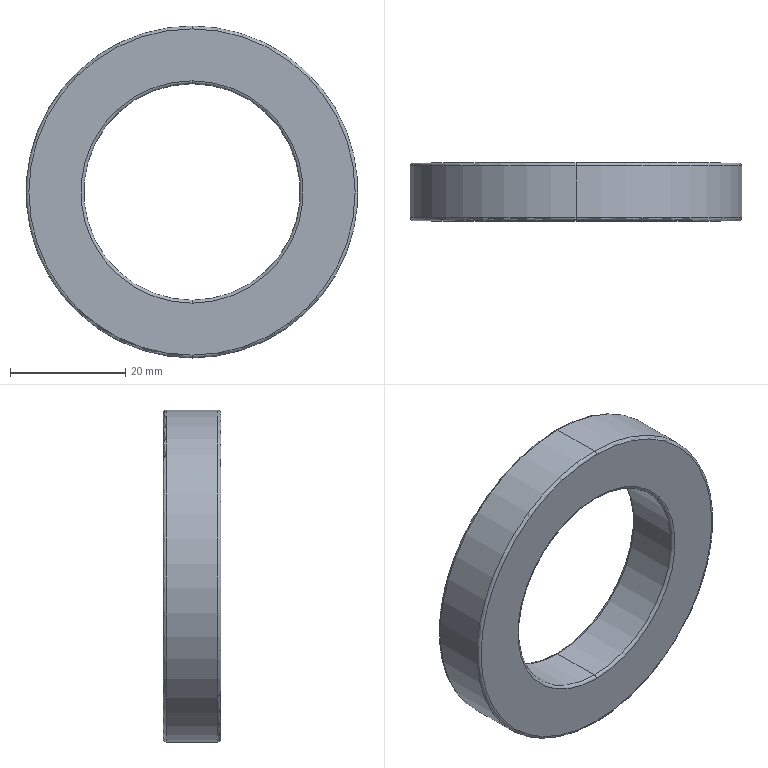Part | STEP file | 2026.6.15-Main Assembly图.sldasm-Part-131 | 1 solid | 14 faces | box 57.5 x 10 x 57.5 mm | volume 14891 mm3 | torus 8 | cylinder 4 | plane 2 | commonest cylinder face diameters 37.5 x2 57.5 x2
STEP:
#1=CARTESIAN_POINT('',(-1589.224,502.551,4179.917));
#2=VERTEX_POINT('',#1);
#3=CARTESIAN_POINT('',(-1589.224,502.551,4237.417));
#4=VERTEX_POINT('',#3);
#5=CARTESIAN_POINT('',(-1589.224,502.551,4208.667));
#6=DIRECTION('',(0.,-1.,0.));
#7=DIRECTION('',(0.,0.,1.));
#8=AXIS2_PLACEMENT_3D('',#5,#6,#7);
#9=CIRCLE('',#8,28.75);
#10=EDGE_CURVE('',#2,#4,#9,.T.);
#11=ORIENTED_EDGE('',*,*,#10,.F.);
#12=CARTESIAN_POINT('',(-1589.224,503.051,4180.417));
#13=VERTEX_POINT('',#12);
#14=CARTESIAN_POINT('',(-1589.224,502.551,4180.417));
#15=DIRECTION('',(1.,0.,0.));
#16=DIRECTION('',(0.,0.,-1.));
#17=AXIS2_PLACEMENT_3D('',#14,#15,#16);
#18=CIRCLE('',#17,0.5);
#19=EDGE_CURVE('',#2,#13,#18,.T.);
#20=ORIENTED_EDGE('',*,*,#19,.T.);
#21=CARTESIAN_POINT('',(-1589.224,503.051,4236.917));
#22=VERTEX_POINT('',#21);
#23=CARTESIAN_POINT('',(-1589.224,503.051,4208.667));
#24=DIRECTION('',(0.,1.,0.));
#25=DIRECTION('',(0.,0.,1.));
#26=AXIS2_PLACEMENT_3D('',#23,#24,#25);
#27=CIRCLE('',#26,28.25);
#28=EDGE_CURVE('',#22,#13,#27,.T.);
#29=ORIENTED_EDGE('',*,*,#28,.F.);
#30=CARTESIAN_POINT('',(-1589.224,502.551,4236.917));
#31=DIRECTION('',(-1.,0.,0.));
#32=DIRECTION('',(0.,0.,1.));
#33=AXIS2_PLACEMENT_3D('',#30,#31,#32);
#34=CIRCLE('',#33,0.5);
#35=EDGE_CURVE('',#4,#22,#34,.T.);
#36=ORIENTED_EDGE('',*,*,#35,.F.);
#37=EDGE_LOOP('',(#11,#20,#29,#36));
#38=FACE_OUTER_BOUND('',#37,.T.);
#39=CARTESIAN_POINT('',(-1589.224,502.551,4208.667));
#40=DIRECTION('',(0.,1.,0.));
#41=DIRECTION('',(0.,0.,1.));
#42=AXIS2_PLACEMENT_3D('',#39,#40,#41);
#43=TOROIDAL_SURFACE('',#42,28.25,0.5);
#44=ADVANCED_FACE('',(#38),#43,.T.);
#45=CARTESIAN_POINT('',(-1589.224,503.051,4189.417));
#46=VERTEX_POINT('',#45);
#47=CARTESIAN_POINT('',(-1589.224,503.051,4227.917));
#48=VERTEX_POINT('',#47);
#49=CARTESIAN_POINT('',(-1589.224,503.051,4208.667));
#50=DIRECTION('',(0.,-1.,0.));
#51=DIRECTION('',(0.,0.,1.));
#52=AXIS2_PLACEMENT_3D('',#49,#50,#51);
#53=CIRCLE('',#52,19.25);
#54=EDGE_CURVE('',#46,#48,#53,.T.);
#55=ORIENTED_EDGE('',*,*,#54,.F.);
#56=CARTESIAN_POINT('',(-1589.224,502.551,4189.917));
#57=VERTEX_POINT('',#56);
#58=CARTESIAN_POINT('',(-1589.224,502.551,4189.417));
#59=DIRECTION('',(1.,0.,0.));
#60=DIRECTION('',(0.,0.,-1.));
#61=AXIS2_PLACEMENT_3D('',#58,#59,#60);
#62=CIRCLE('',#61,0.5);
#63=EDGE_CURVE('',#46,#57,#62,.T.);
#64=ORIENTED_EDGE('',*,*,#63,.T.);
#65=CARTESIAN_POINT('',(-1589.224,502.551,4227.417));
#66=VERTEX_POINT('',#65);
#67=CARTESIAN_POINT('',(-1589.224,502.551,4208.667));
#68=DIRECTION('',(0.,1.,0.));
#69=DIRECTION('',(0.,0.,1.));
#70=AXIS2_PLACEMENT_3D('',#67,#68,#69);
#71=CIRCLE('',#70,18.75);
#72=EDGE_CURVE('',#66,#57,#71,.T.);
#73=ORIENTED_EDGE('',*,*,#72,.F.);
#74=CARTESIAN_POINT('',(-1589.224,502.551,4227.917));
#75=DIRECTION('',(-1.,0.,0.));
#76=DIRECTION('',(0.,0.,1.));
#77=AXIS2_PLACEMENT_3D('',#74,#75,#76);
#78=CIRCLE('',#77,0.5);
#79=EDGE_CURVE('',#48,#66,#78,.T.);
#80=ORIENTED_EDGE('',*,*,#79,.F.);
#81=EDGE_LOOP('',(#55,#64,#73,#80));
#82=FACE_OUTER_BOUND('',#81,.T.);
#83=CARTESIAN_POINT('',(-1589.224,502.551,4208.667));
#84=DIRECTION('',(0.,1.,0.));
#85=DIRECTION('',(0.,0.,1.));
#86=AXIS2_PLACEMENT_3D('',#83,#84,#85);
#87=TOROIDAL_SURFACE('',#86,19.25,0.5);
#88=ADVANCED_FACE('',(#82),#87,.T.);
#89=CARTESIAN_POINT('',(-1589.224,493.051,4227.917));
#90=VERTEX_POINT('',#89);
#91=CARTESIAN_POINT('',(-1589.224,493.051,4189.417));
#92=VERTEX_POINT('',#91);
#93=CARTESIAN_POINT('',(-1589.224,493.051,4208.667));
#94=DIRECTION('',(0.,1.,0.));
#95=DIRECTION('',(0.,0.,-1.));
#96=AXIS2_PLACEMENT_3D('',#93,#94,#95);
#97=CIRCLE('',#96,19.25);
#98=EDGE_CURVE('',#90,#92,#97,.T.);
#99=ORIENTED_EDGE('',*,*,#98,.F.);
#100=CARTESIAN_POINT('',(-1589.224,493.551,4227.417));
#101=VERTEX_POINT('',#100);
#102=CARTESIAN_POINT('',(-1589.224,493.551,4227.917));
#103=DIRECTION('',(1.,0.,0.));
#104=DIRECTION('',(0.,0.,-1.));
#105=AXIS2_PLACEMENT_3D('',#102,#103,#104);
#106=CIRCLE('',#105,0.5);
#107=EDGE_CURVE('',#90,#101,#106,.T.);
#108=ORIENTED_EDGE('',*,*,#107,.T.);
#109=CARTESIAN_POINT('',(-1589.224,493.551,4189.917));
#110=VERTEX_POINT('',#109);
#111=CARTESIAN_POINT('',(-1589.224,493.551,4208.667));
#112=DIRECTION('',(0.,-1.,0.));
#113=DIRECTION('',(0.,0.,-1.));
#114=AXIS2_PLACEMENT_3D('',#111,#112,#113);
#115=CIRCLE('',#114,18.75);
#116=EDGE_CURVE('',#110,#101,#115,.T.);
#117=ORIENTED_EDGE('',*,*,#116,.F.);
#118=CARTESIAN_POINT('',(-1589.224,493.551,4189.417));
#119=DIRECTION('',(-1.,0.,0.));
#120=DIRECTION('',(0.,0.,1.));
#121=AXIS2_PLACEMENT_3D('',#118,#119,#120);
#122=CIRCLE('',#121,0.5);
#123=EDGE_CURVE('',#92,#110,#122,.T.);
#124=ORIENTED_EDGE('',*,*,#123,.F.);
#125=EDGE_LOOP('',(#99,#108,#117,#124));
#126=FACE_OUTER_BOUND('',#125,.T.);
#127=CARTESIAN_POINT('',(-1589.224,493.551,4208.667));
#128=DIRECTION('',(0.,-1.,0.));
#129=DIRECTION('',(0.,0.,-1.));
#130=AXIS2_PLACEMENT_3D('',#127,#128,#129);
#131=TOROIDAL_SURFACE('',#130,19.25,0.5);
#132=ADVANCED_FACE('',(#126),#131,.T.);
#133=CARTESIAN_POINT('',(-1589.224,493.551,4237.417));
#134=VERTEX_POINT('',#133);
#135=CARTESIAN_POINT('',(-1589.224,493.551,4179.917));
#136=VERTEX_POINT('',#135);
#137=CARTESIAN_POINT('',(-1589.224,493.551,4208.667));
#138=DIRECTION('',(0.,1.,0.));
#139=DIRECTION('',(0.,0.,-1.));
#140=AXIS2_PLACEMENT_3D('',#137,#138,#139);
#141=CIRCLE('',#140,28.75);
#142=EDGE_CURVE('',#134,#136,#141,.T.);
#143=ORIENTED_EDGE('',*,*,#142,.F.);
#144=CARTESIAN_POINT('',(-1589.224,493.051,4236.917));
#145=VERTEX_POINT('',#144);
#146=CARTESIAN_POINT('',(-1589.224,493.551,4236.917));
#147=DIRECTION('',(1.,0.,0.));
#148=DIRECTION('',(0.,0.,-1.));
#149=AXIS2_PLACEMENT_3D('',#146,#147,#148);
#150=CIRCLE('',#149,0.5);
#151=EDGE_CURVE('',#134,#145,#150,.T.);
#152=ORIENTED_EDGE('',*,*,#151,.T.);
#153=CARTESIAN_POINT('',(-1589.224,493.051,4180.417));
#154=VERTEX_POINT('',#153);
#155=CARTESIAN_POINT('',(-1589.224,493.051,4208.667));
#156=DIRECTION('',(0.,-1.,0.));
#157=DIRECTION('',(0.,0.,-1.));
#158=AXIS2_PLACEMENT_3D('',#155,#156,#157);
#159=CIRCLE('',#158,28.25);
#160=EDGE_CURVE('',#154,#145,#159,.T.);
#161=ORIENTED_EDGE('',*,*,#160,.F.);
#162=CARTESIAN_POINT('',(-1589.224,493.551,4180.417));
#163=DIRECTION('',(-1.,0.,0.));
#164=DIRECTION('',(0.,0.,1.));
#165=AXIS2_PLACEMENT_3D('',#162,#163,#164);
#166=CIRCLE('',#165,0.5);
#167=EDGE_CURVE('',#136,#154,#166,.T.);
#168=ORIENTED_EDGE('',*,*,#167,.F.);
#169=EDGE_LOOP('',(#143,#152,#161,#168));
#170=FACE_OUTER_BOUND('',#169,.T.);
#171=CARTESIAN_POINT('',(-1589.224,493.551,4208.667));
#172=DIRECTION('',(0.,-1.,0.));
#173=DIRECTION('',(0.,0.,-1.));
#174=AXIS2_PLACEMENT_3D('',#171,#172,#173);
#175=TOROIDAL_SURFACE('',#174,28.25,0.5);
#176=ADVANCED_FACE('',(#170),#175,.T.);
#177=CARTESIAN_POINT('',(-1589.224,493.551,4208.667));
#178=DIRECTION('',(0.,-1.,0.));
#179=DIRECTION('',(0.,0.,-1.));
#180=AXIS2_PLACEMENT_3D('',#177,#178,#179);
#181=CIRCLE('',#180,18.75);
#182=EDGE_CURVE('',#101,#110,#181,.T.);
#183=ORIENTED_EDGE('',*,*,#182,.T.);
#184=CARTESIAN_POINT('',(-1589.224,493.051,4189.917));
#185=DIRECTION('',(0.,1.,0.));
#186=VECTOR('',#185,1000.);
#187=LINE('',#184,#186);
#188=EDGE_CURVE('',#110,#57,#187,.T.);
#189=ORIENTED_EDGE('',*,*,#188,.T.);
#190=CARTESIAN_POINT('',(-1589.224,502.551,4208.667));
#191=DIRECTION('',(0.,1.,0.));
#192=DIRECTION('',(0.,0.,1.));
#193=AXIS2_PLACEMENT_3D('',#190,#191,#192);
#194=CIRCLE('',#193,18.75);
#195=EDGE_CURVE('',#57,#66,#194,.T.);
#196=ORIENTED_EDGE('',*,*,#195,.T.);
#197=CARTESIAN_POINT('',(-1589.224,493.051,4227.417));
#198=DIRECTION('',(0.,1.,0.));
#199=VECTOR('',#198,1000.);
#200=LINE('',#197,#199);
#201=EDGE_CURVE('',#101,#66,#200,.T.);
#202=ORIENTED_EDGE('',*,*,#201,.F.);
#203=EDGE_LOOP('',(#183,#189,#196,#202));
#204=FACE_OUTER_BOUND('',#203,.T.);
#205=CARTESIAN_POINT('',(-1589.224,493.051,4208.667));
#206=DIRECTION('',(0.,1.,0.));
#207=DIRECTION('',(0.,0.,1.));
#208=AXIS2_PLACEMENT_3D('',#205,#206,#207);
#209=CYLINDRICAL_SURFACE('',#208,18.75);
#210=ADVANCED_FACE('',(#204),#209,.F.);
#211=ORIENTED_EDGE('',*,*,#142,.T.);
#212=CARTESIAN_POINT('',(-1589.224,493.051,4179.917));
#213=DIRECTION('',(0.,1.,0.));
#214=VECTOR('',#213,1000.);
#215=LINE('',#212,#214);
#216=EDGE_CURVE('',#136,#2,#215,.T.);
#217=ORIENTED_EDGE('',*,*,#216,.T.);
#218=ORIENTED_EDGE('',*,*,#10,.T.);
#219=CARTESIAN_POINT('',(-1589.224,493.051,4237.417));
#220=DIRECTION('',(0.,1.,0.));
#221=VECTOR('',#220,1000.);
#222=LINE('',#219,#221);
#223=EDGE_CURVE('',#134,#4,#222,.T.);
#224=ORIENTED_EDGE('',*,*,#223,.F.);
#225=EDGE_LOOP('',(#211,#217,#218,#224));
#226=FACE_OUTER_BOUND('',#225,.T.);
#227=CARTESIAN_POINT('',(-1589.224,493.051,4208.667));
#228=DIRECTION('',(0.,1.,0.));
#229=DIRECTION('',(0.,0.,1.));
#230=AXIS2_PLACEMENT_3D('',#227,#228,#229);
#231=CYLINDRICAL_SURFACE('',#230,28.75);
#232=ADVANCED_FACE('',(#226),#231,.T.);
#233=CARTESIAN_POINT('',(-1589.224,503.051,4208.667));
#234=DIRECTION('',(0.,-1.,0.));
#235=DIRECTION('',(0.,0.,1.));
#236=AXIS2_PLACEMENT_3D('',#233,#234,#235);
#237=CIRCLE('',#236,19.25);
#238=EDGE_CURVE('',#48,#46,#237,.T.);
#239=ORIENTED_EDGE('',*,*,#238,.T.);
#240=ORIENTED_EDGE('',*,*,#54,.T.);
#241=EDGE_LOOP('',(#239,#240));
#242=FACE_BOUND('',#241,.T.);
#243=ORIENTED_EDGE('',*,*,#28,.T.);
#244=CARTESIAN_POINT('',(-1589.224,503.051,4208.667));
#245=DIRECTION('',(0.,1.,0.));
#246=DIRECTION('',(0.,0.,1.));
#247=AXIS2_PLACEMENT_3D('',#244,#245,#246);
#248=CIRCLE('',#247,28.25);
#249=EDGE_CURVE('',#13,#22,#248,.T.);
#250=ORIENTED_EDGE('',*,*,#249,.T.);
#251=EDGE_LOOP('',(#243,#250));
#252=FACE_OUTER_BOUND('',#251,.T.);
#253=CARTESIAN_POINT('',(-1589.224,503.051,4208.667));
#254=DIRECTION('',(0.,1.,0.));
#255=DIRECTION('',(0.,0.,1.));
#256=AXIS2_PLACEMENT_3D('',#253,#254,#255);
#257=PLANE('',#256);
#258=ADVANCED_FACE('',(#242,#252),#257,.T.);
#259=ORIENTED_EDGE('',*,*,#160,.T.);
#260=CARTESIAN_POINT('',(-1589.224,493.051,4208.667));
#261=DIRECTION('',(0.,-1.,0.));
#262=DIRECTION('',(0.,0.,-1.));
#263=AXIS2_PLACEMENT_3D('',#260,#261,#262);
#264=CIRCLE('',#263,28.25);
#265=EDGE_CURVE('',#145,#154,#264,.T.);
#266=ORIENTED_EDGE('',*,*,#265,.T.);
#267=EDGE_LOOP('',(#259,#266));
#268=FACE_OUTER_BOUND('',#267,.T.);
#269=CARTESIAN_POINT('',(-1589.224,493.051,4208.667));
#270=DIRECTION('',(0.,1.,0.));
#271=DIRECTION('',(0.,0.,-1.));
#272=AXIS2_PLACEMENT_3D('',#269,#270,#271);
#273=CIRCLE('',#272,19.25);
#274=EDGE_CURVE('',#92,#90,#273,.T.);
#275=ORIENTED_EDGE('',*,*,#274,.T.);
#276=ORIENTED_EDGE('',*,*,#98,.T.);
#277=EDGE_LOOP('',(#275,#276));
#278=FACE_BOUND('',#277,.T.);
#279=CARTESIAN_POINT('',(-1589.224,493.051,4208.667));
#280=DIRECTION('',(0.,-1.,0.));
#281=DIRECTION('',(0.,0.,-1.));
#282=AXIS2_PLACEMENT_3D('',#279,#280,#281);
#283=PLANE('',#282);
#284=ADVANCED_FACE('',(#268,#278),#283,.T.);
#285=ORIENTED_EDGE('',*,*,#216,.F.);
#286=CARTESIAN_POINT('',(-1589.224,493.551,4208.667));
#287=DIRECTION('',(0.,1.,0.));
#288=DIRECTION('',(0.,0.,-1.));
#289=AXIS2_PLACEMENT_3D('',#286,#287,#288);
#290=CIRCLE('',#289,28.75);
#291=EDGE_CURVE('',#136,#134,#290,.T.);
#292=ORIENTED_EDGE('',*,*,#291,.T.);
#293=ORIENTED_EDGE('',*,*,#223,.T.);
#294=CARTESIAN_POINT('',(-1589.224,502.551,4208.667));
#295=DIRECTION('',(0.,-1.,0.));
#296=DIRECTION('',(0.,0.,1.));
#297=AXIS2_PLACEMENT_3D('',#294,#295,#296);
#298=CIRCLE('',#297,28.75);
#299=EDGE_CURVE('',#4,#2,#298,.T.);
#300=ORIENTED_EDGE('',*,*,#299,.T.);
#301=EDGE_LOOP('',(#285,#292,#293,#300));
#302=FACE_OUTER_BOUND('',#301,.T.);
#303=CARTESIAN_POINT('',(-1589.224,493.051,4208.667));
#304=DIRECTION('',(0.,1.,0.));
#305=DIRECTION('',(0.,0.,1.));
#306=AXIS2_PLACEMENT_3D('',#303,#304,#305);
#307=CYLINDRICAL_SURFACE('',#306,28.75);
#308=ADVANCED_FACE('',(#302),#307,.T.);
#309=ORIENTED_EDGE('',*,*,#188,.F.);
#310=ORIENTED_EDGE('',*,*,#116,.T.);
#311=ORIENTED_EDGE('',*,*,#201,.T.);
#312=ORIENTED_EDGE('',*,*,#72,.T.);
#313=EDGE_LOOP('',(#309,#310,#311,#312));
#314=FACE_OUTER_BOUND('',#313,.T.);
#315=CARTESIAN_POINT('',(-1589.224,493.051,4208.667));
#316=DIRECTION('',(0.,1.,0.));
#317=DIRECTION('',(0.,0.,1.));
#318=AXIS2_PLACEMENT_3D('',#315,#316,#317);
#319=CYLINDRICAL_SURFACE('',#318,18.75);
#320=ADVANCED_FACE('',(#314),#319,.F.);
#321=ORIENTED_EDGE('',*,*,#151,.F.);
#322=ORIENTED_EDGE('',*,*,#291,.F.);
#323=ORIENTED_EDGE('',*,*,#167,.T.);
#324=ORIENTED_EDGE('',*,*,#265,.F.);
#325=EDGE_LOOP('',(#321,#322,#323,#324));
#326=FACE_OUTER_BOUND('',#325,.T.);
#327=CARTESIAN_POINT('',(-1589.224,493.551,4208.667));
#328=DIRECTION('',(0.,-1.,0.));
#329=DIRECTION('',(0.,0.,-1.));
#330=AXIS2_PLACEMENT_3D('',#327,#328,#329);
#331=TOROIDAL_SURFACE('',#330,28.25,0.5);
#332=ADVANCED_FACE('',(#326),#331,.T.);
#333=ORIENTED_EDGE('',*,*,#107,.F.);
#334=ORIENTED_EDGE('',*,*,#274,.F.);
#335=ORIENTED_EDGE('',*,*,#123,.T.);
#336=ORIENTED_EDGE('',*,*,#182,.F.);
#337=EDGE_LOOP('',(#333,#334,#335,#336));
#338=FACE_OUTER_BOUND('',#337,.T.);
#339=CARTESIAN_POINT('',(-1589.224,493.551,4208.667));
#340=DIRECTION('',(0.,-1.,0.));
#341=DIRECTION('',(0.,0.,-1.));
#342=AXIS2_PLACEMENT_3D('',#339,#340,#341);
#343=TOROIDAL_SURFACE('',#342,19.25,0.5);
#344=ADVANCED_FACE('',(#338),#343,.T.);
#345=ORIENTED_EDGE('',*,*,#63,.F.);
#346=ORIENTED_EDGE('',*,*,#238,.F.);
#347=ORIENTED_EDGE('',*,*,#79,.T.);
#348=ORIENTED_EDGE('',*,*,#195,.F.);
#349=EDGE_LOOP('',(#345,#346,#347,#348));
#350=FACE_OUTER_BOUND('',#349,.T.);
#351=CARTESIAN_POINT('',(-1589.224,502.551,4208.667));
#352=DIRECTION('',(0.,1.,0.));
#353=DIRECTION('',(0.,0.,1.));
#354=AXIS2_PLACEMENT_3D('',#351,#352,#353);
#355=TOROIDAL_SURFACE('',#354,19.25,0.5);
#356=ADVANCED_FACE('',(#350),#355,.T.);
#357=ORIENTED_EDGE('',*,*,#19,.F.);
#358=ORIENTED_EDGE('',*,*,#299,.F.);
#359=ORIENTED_EDGE('',*,*,#35,.T.);
#360=ORIENTED_EDGE('',*,*,#249,.F.);
#361=EDGE_LOOP('',(#357,#358,#359,#360));
#362=FACE_OUTER_BOUND('',#361,.T.);
#363=CARTESIAN_POINT('',(-1589.224,502.551,4208.667));
#364=DIRECTION('',(0.,1.,0.));
#365=DIRECTION('',(0.,0.,1.));
#366=AXIS2_PLACEMENT_3D('',#363,#364,#365);
#367=TOROIDAL_SURFACE('',#366,28.25,0.5);
#368=ADVANCED_FACE('',(#362),#367,.T.);
#369=CLOSED_SHELL('',(#44,#88,#132,#176,#210,#232,#258,#284,#308,#320,#332,#344,#356,#368));
#370=MANIFOLD_SOLID_BREP('',#369);
#371=CARTESIAN_POINT('',(0.,0.,0.));
#372=DIRECTION('',(0.,0.,1.));
#373=DIRECTION('',(1.,0.,0.));
#374=AXIS2_PLACEMENT_3D('',#371,#372,#373);
#375=(LENGTH_UNIT()NAMED_UNIT(*)SI_UNIT(.MILLI.,.METRE.));
#376=UNCERTAINTY_MEASURE_WITH_UNIT(LENGTH_MEASURE(0.00001),#375,'','');
#377=(NAMED_UNIT(*)PLANE_ANGLE_UNIT()SI_UNIT($,.RADIAN.));
#378=(NAMED_UNIT(*)SI_UNIT($,.STERADIAN.)SOLID_ANGLE_UNIT());
#379=(GEOMETRIC_REPRESENTATION_CONTEXT(3)GLOBAL_UNCERTAINTY_ASSIGNED_CONTEXT((#376))GLOBAL_UNIT_ASSIGNED_CONTEXT((#375,#377,#378))REPRESENTATION_CONTEXT('',''));
#380=ADVANCED_BREP_SHAPE_REPRESENTATION('',(#370,#374),#379);